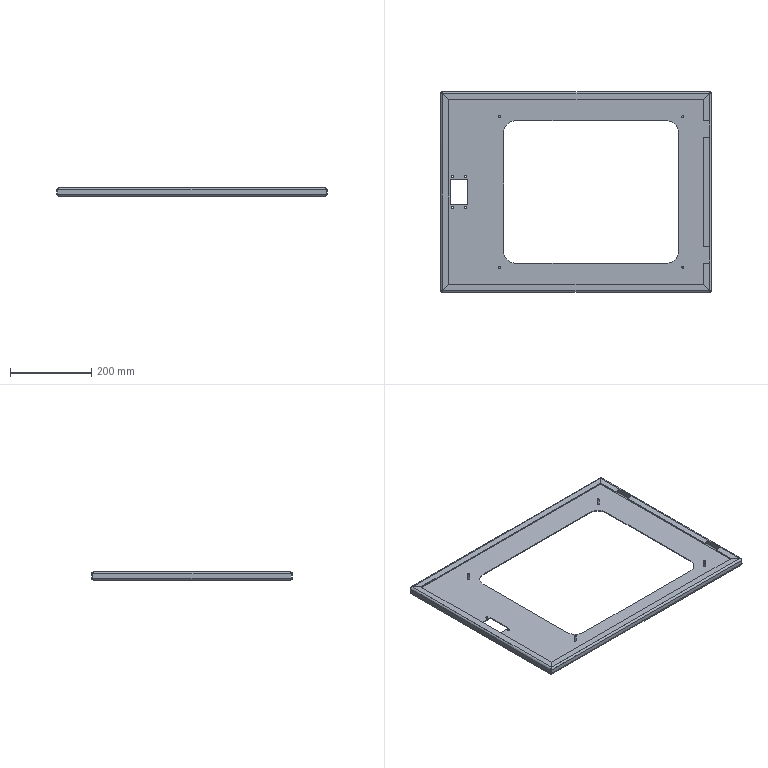Part | SolidWorks | features Cut 3, ICE 2, Fillet 1, FlatPattern 1, MirrorPattern 1, SMBaseFlange 1, SMMiteredFlange 1, SheetMetal 1 | 1 solid | 114 faces | box 664.5 x 493 x 20 mm | volume 495886 mm3 | plane 62 | cylinder 36 | spline 16 | commonest cylinder face diameters 5 x16 6 x8 10 x8 60 x4